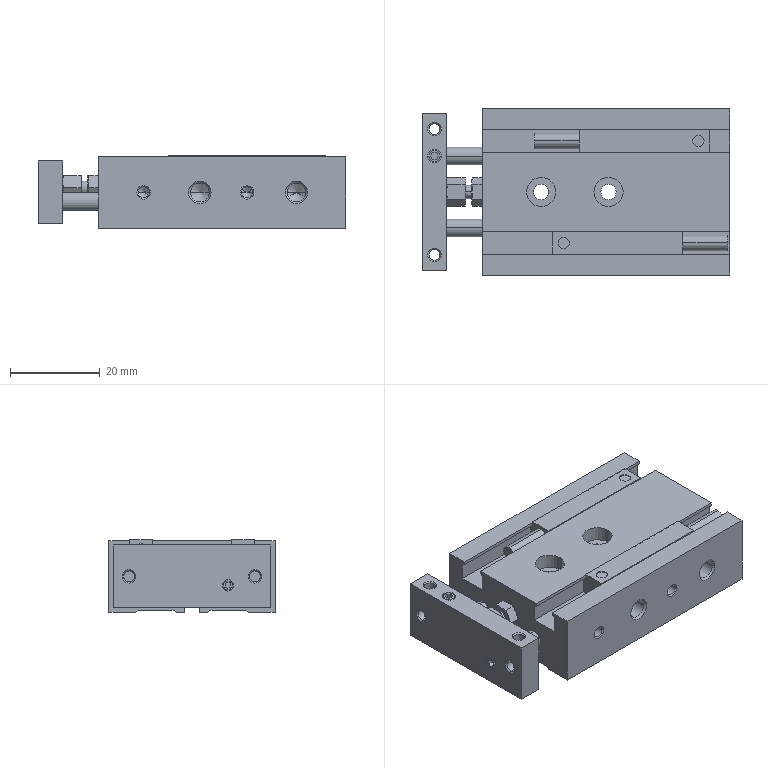Part | SolidWorks | features AEMSimFeature 1 | 4 solids | 277 faces | box 68.5 x 37 x 16.2 mm | volume 31090 mm3 | plane 115 | cylinder 82 | cone 80 | commonest cylinder face diameters 2.459 x24 3.4 x12 4.134 x12 2.5 x8 4 x8 6 x8